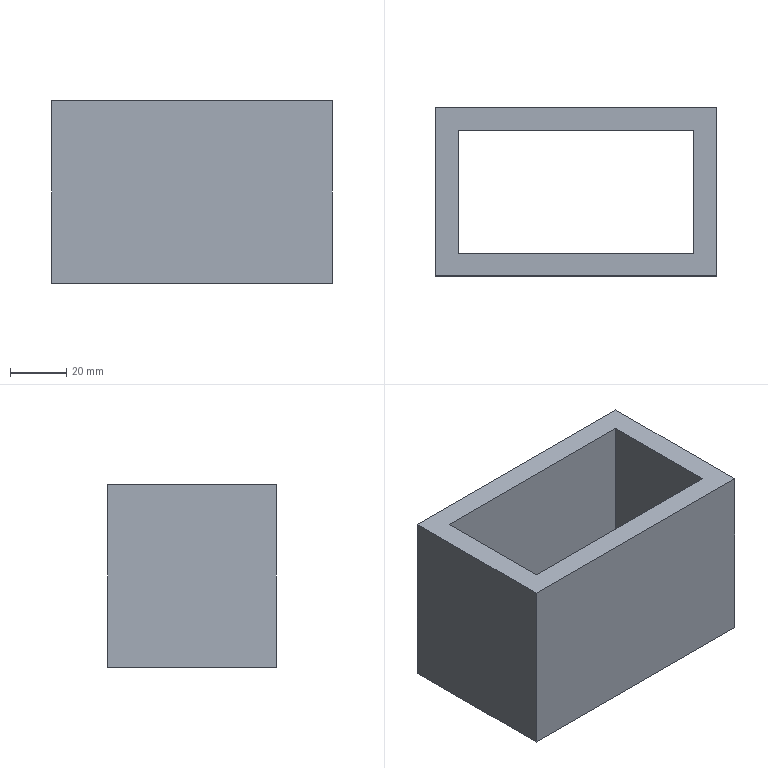Part | SolidWorks | features BaseBody 1 | 1 solid | 10 faces | box 100 x 60 x 65 mm | volume 149760 mm3 | plane 10
STEP:
#1=CARTESIAN_POINT('',(-50.,-30.,32.5));
#2=VERTEX_POINT('',#1);
#3=CARTESIAN_POINT('',(50.,-30.,32.5));
#4=VERTEX_POINT('',#3);
#5=CARTESIAN_POINT('',(-50.,-30.,32.5));
#6=DIRECTION('',(1.,0.,0.));
#7=VECTOR('',#6,1000.);
#8=LINE('',#5,#7);
#9=EDGE_CURVE('',#2,#4,#8,.T.);
#10=ORIENTED_EDGE('',*,*,#9,.F.);
#11=CARTESIAN_POINT('',(-50.,-30.,-32.5));
#12=VERTEX_POINT('',#11);
#13=CARTESIAN_POINT('',(-50.,-30.,-32.5));
#14=DIRECTION('',(0.,0.,1.));
#15=VECTOR('',#14,1000.);
#16=LINE('',#13,#15);
#17=EDGE_CURVE('',#12,#2,#16,.T.);
#18=ORIENTED_EDGE('',*,*,#17,.F.);
#19=CARTESIAN_POINT('',(50.,-30.,-32.5));
#20=VERTEX_POINT('',#19);
#21=CARTESIAN_POINT('',(-50.,-30.,-32.5));
#22=DIRECTION('',(-1.,0.,0.));
#23=VECTOR('',#22,1000.);
#24=LINE('',#21,#23);
#25=EDGE_CURVE('',#20,#12,#24,.T.);
#26=ORIENTED_EDGE('',*,*,#25,.F.);
#27=CARTESIAN_POINT('',(50.,-30.,-32.5));
#28=DIRECTION('',(0.,0.,-1.));
#29=VECTOR('',#28,1000.);
#30=LINE('',#27,#29);
#31=EDGE_CURVE('',#4,#20,#30,.T.);
#32=ORIENTED_EDGE('',*,*,#31,.F.);
#33=EDGE_LOOP('',(#10,#18,#26,#32));
#34=FACE_OUTER_BOUND('',#33,.T.);
#35=CARTESIAN_POINT('',(-50.,-30.,-32.5));
#36=DIRECTION('',(0.,1.,0.));
#37=DIRECTION('',(0.,0.,1.));
#38=AXIS2_PLACEMENT_3D('',#35,#36,#37);
#39=PLANE('',#38);
#40=ADVANCED_FACE('',(#34),#39,.F.);
#41=CARTESIAN_POINT('',(50.,30.,-32.5));
#42=VERTEX_POINT('',#41);
#43=CARTESIAN_POINT('',(50.,30.,32.5));
#44=VERTEX_POINT('',#43);
#45=CARTESIAN_POINT('',(50.,30.,-32.5));
#46=DIRECTION('',(0.,0.,1.));
#47=VECTOR('',#46,1000.);
#48=LINE('',#45,#47);
#49=EDGE_CURVE('',#42,#44,#48,.T.);
#50=ORIENTED_EDGE('',*,*,#49,.T.);
#51=CARTESIAN_POINT('',(50.,-30.,32.5));
#52=DIRECTION('',(0.,-1.,0.));
#53=VECTOR('',#52,1000.);
#54=LINE('',#51,#53);
#55=EDGE_CURVE('',#44,#4,#54,.T.);
#56=ORIENTED_EDGE('',*,*,#55,.T.);
#57=ORIENTED_EDGE('',*,*,#31,.T.);
#58=CARTESIAN_POINT('',(50.,-30.,-32.5));
#59=DIRECTION('',(0.,1.,0.));
#60=VECTOR('',#59,1000.);
#61=LINE('',#58,#60);
#62=EDGE_CURVE('',#20,#42,#61,.T.);
#63=ORIENTED_EDGE('',*,*,#62,.T.);
#64=EDGE_LOOP('',(#50,#56,#57,#63));
#65=FACE_OUTER_BOUND('',#64,.T.);
#66=CARTESIAN_POINT('',(50.,-30.,-32.5));
#67=DIRECTION('',(1.,0.,0.));
#68=DIRECTION('',(0.,0.,-1.));
#69=AXIS2_PLACEMENT_3D('',#66,#67,#68);
#70=PLANE('',#69);
#71=ADVANCED_FACE('',(#65),#70,.T.);
#72=CARTESIAN_POINT('',(-42.,22.,32.5));
#73=VERTEX_POINT('',#72);
#74=CARTESIAN_POINT('',(42.,22.,32.5));
#75=VERTEX_POINT('',#74);
#76=CARTESIAN_POINT('',(-50.,22.,32.5));
#77=DIRECTION('',(1.,0.,0.));
#78=VECTOR('',#77,1000.);
#79=LINE('',#76,#78);
#80=EDGE_CURVE('',#73,#75,#79,.T.);
#81=ORIENTED_EDGE('',*,*,#80,.T.);
#82=CARTESIAN_POINT('',(42.,-22.,32.5));
#83=VERTEX_POINT('',#82);
#84=CARTESIAN_POINT('',(42.,-30.,32.5));
#85=DIRECTION('',(0.,-1.,0.));
#86=VECTOR('',#85,1000.);
#87=LINE('',#84,#86);
#88=EDGE_CURVE('',#75,#83,#87,.T.);
#89=ORIENTED_EDGE('',*,*,#88,.T.);
#90=CARTESIAN_POINT('',(-42.,-22.,32.5));
#91=VERTEX_POINT('',#90);
#92=CARTESIAN_POINT('',(-50.,-22.,32.5));
#93=DIRECTION('',(-1.,0.,0.));
#94=VECTOR('',#93,1000.);
#95=LINE('',#92,#94);
#96=EDGE_CURVE('',#83,#91,#95,.T.);
#97=ORIENTED_EDGE('',*,*,#96,.T.);
#98=CARTESIAN_POINT('',(-42.,-30.,32.5));
#99=DIRECTION('',(0.,1.,0.));
#100=VECTOR('',#99,1000.);
#101=LINE('',#98,#100);
#102=EDGE_CURVE('',#91,#73,#101,.T.);
#103=ORIENTED_EDGE('',*,*,#102,.T.);
#104=EDGE_LOOP('',(#81,#89,#97,#103));
#105=FACE_BOUND('',#104,.T.);
#106=ORIENTED_EDGE('',*,*,#55,.F.);
#107=CARTESIAN_POINT('',(-50.,30.,32.5));
#108=VERTEX_POINT('',#107);
#109=CARTESIAN_POINT('',(-50.,30.,32.5));
#110=DIRECTION('',(-1.,0.,0.));
#111=VECTOR('',#110,1000.);
#112=LINE('',#109,#111);
#113=EDGE_CURVE('',#44,#108,#112,.T.);
#114=ORIENTED_EDGE('',*,*,#113,.T.);
#115=CARTESIAN_POINT('',(-50.,-30.,32.5));
#116=DIRECTION('',(0.,-1.,0.));
#117=VECTOR('',#116,1000.);
#118=LINE('',#115,#117);
#119=EDGE_CURVE('',#108,#2,#118,.T.);
#120=ORIENTED_EDGE('',*,*,#119,.T.);
#121=ORIENTED_EDGE('',*,*,#9,.T.);
#122=EDGE_LOOP('',(#106,#114,#120,#121));
#123=FACE_OUTER_BOUND('',#122,.T.);
#124=CARTESIAN_POINT('',(-50.,-30.,32.5));
#125=DIRECTION('',(0.,0.,1.));
#126=DIRECTION('',(1.,0.,0.));
#127=AXIS2_PLACEMENT_3D('',#124,#125,#126);
#128=PLANE('',#127);
#129=ADVANCED_FACE('',(#105,#123),#128,.T.);
#130=CARTESIAN_POINT('',(-50.,30.,-32.5));
#131=VERTEX_POINT('',#130);
#132=CARTESIAN_POINT('',(-50.,30.,-32.5));
#133=DIRECTION('',(0.,0.,1.));
#134=VECTOR('',#133,1000.);
#135=LINE('',#132,#134);
#136=EDGE_CURVE('',#131,#108,#135,.T.);
#137=ORIENTED_EDGE('',*,*,#136,.F.);
#138=CARTESIAN_POINT('',(-50.,-30.,-32.5));
#139=DIRECTION('',(0.,1.,0.));
#140=VECTOR('',#139,1000.);
#141=LINE('',#138,#140);
#142=EDGE_CURVE('',#12,#131,#141,.T.);
#143=ORIENTED_EDGE('',*,*,#142,.F.);
#144=ORIENTED_EDGE('',*,*,#17,.T.);
#145=ORIENTED_EDGE('',*,*,#119,.F.);
#146=EDGE_LOOP('',(#137,#143,#144,#145));
#147=FACE_OUTER_BOUND('',#146,.T.);
#148=CARTESIAN_POINT('',(-50.,-30.,-32.5));
#149=DIRECTION('',(1.,0.,0.));
#150=DIRECTION('',(0.,0.,-1.));
#151=AXIS2_PLACEMENT_3D('',#148,#149,#150);
#152=PLANE('',#151);
#153=ADVANCED_FACE('',(#147),#152,.F.);
#154=CARTESIAN_POINT('',(-42.,22.,-32.5));
#155=VERTEX_POINT('',#154);
#156=CARTESIAN_POINT('',(42.,22.,-32.5));
#157=VERTEX_POINT('',#156);
#158=CARTESIAN_POINT('',(-50.,22.,-32.5));
#159=DIRECTION('',(1.,0.,0.));
#160=VECTOR('',#159,1000.);
#161=LINE('',#158,#160);
#162=EDGE_CURVE('',#155,#157,#161,.T.);
#163=ORIENTED_EDGE('',*,*,#162,.F.);
#164=CARTESIAN_POINT('',(-42.,-22.,-32.5));
#165=VERTEX_POINT('',#164);
#166=CARTESIAN_POINT('',(-42.,-30.,-32.5));
#167=DIRECTION('',(0.,1.,0.));
#168=VECTOR('',#167,1000.);
#169=LINE('',#166,#168);
#170=EDGE_CURVE('',#165,#155,#169,.T.);
#171=ORIENTED_EDGE('',*,*,#170,.F.);
#172=CARTESIAN_POINT('',(42.,-22.,-32.5));
#173=VERTEX_POINT('',#172);
#174=CARTESIAN_POINT('',(-50.,-22.,-32.5));
#175=DIRECTION('',(-1.,0.,0.));
#176=VECTOR('',#175,1000.);
#177=LINE('',#174,#176);
#178=EDGE_CURVE('',#173,#165,#177,.T.);
#179=ORIENTED_EDGE('',*,*,#178,.F.);
#180=CARTESIAN_POINT('',(42.,-30.,-32.5));
#181=DIRECTION('',(0.,-1.,0.));
#182=VECTOR('',#181,1000.);
#183=LINE('',#180,#182);
#184=EDGE_CURVE('',#157,#173,#183,.T.);
#185=ORIENTED_EDGE('',*,*,#184,.F.);
#186=EDGE_LOOP('',(#163,#171,#179,#185));
#187=FACE_BOUND('',#186,.T.);
#188=ORIENTED_EDGE('',*,*,#62,.F.);
#189=ORIENTED_EDGE('',*,*,#25,.T.);
#190=ORIENTED_EDGE('',*,*,#142,.T.);
#191=CARTESIAN_POINT('',(-50.,30.,-32.5));
#192=DIRECTION('',(-1.,0.,0.));
#193=VECTOR('',#192,1000.);
#194=LINE('',#191,#193);
#195=EDGE_CURVE('',#42,#131,#194,.T.);
#196=ORIENTED_EDGE('',*,*,#195,.F.);
#197=EDGE_LOOP('',(#188,#189,#190,#196));
#198=FACE_OUTER_BOUND('',#197,.T.);
#199=CARTESIAN_POINT('',(-50.,-30.,-32.5));
#200=DIRECTION('',(0.,0.,1.));
#201=DIRECTION('',(1.,0.,0.));
#202=AXIS2_PLACEMENT_3D('',#199,#200,#201);
#203=PLANE('',#202);
#204=ADVANCED_FACE('',(#187,#198),#203,.F.);
#205=ORIENTED_EDGE('',*,*,#113,.F.);
#206=ORIENTED_EDGE('',*,*,#49,.F.);
#207=ORIENTED_EDGE('',*,*,#195,.T.);
#208=ORIENTED_EDGE('',*,*,#136,.T.);
#209=EDGE_LOOP('',(#205,#206,#207,#208));
#210=FACE_OUTER_BOUND('',#209,.T.);
#211=CARTESIAN_POINT('',(-50.,30.,-32.5));
#212=DIRECTION('',(0.,1.,0.));
#213=DIRECTION('',(0.,0.,1.));
#214=AXIS2_PLACEMENT_3D('',#211,#212,#213);
#215=PLANE('',#214);
#216=ADVANCED_FACE('',(#210),#215,.T.);
#217=CARTESIAN_POINT('',(42.,22.,-33.5));
#218=DIRECTION('',(0.,0.,1.));
#219=VECTOR('',#218,1000.);
#220=LINE('',#217,#219);
#221=EDGE_CURVE('',#157,#75,#220,.T.);
#222=ORIENTED_EDGE('',*,*,#221,.F.);
#223=ORIENTED_EDGE('',*,*,#184,.T.);
#224=CARTESIAN_POINT('',(42.,-22.,-33.5));
#225=DIRECTION('',(0.,0.,-1.));
#226=VECTOR('',#225,1000.);
#227=LINE('',#224,#226);
#228=EDGE_CURVE('',#83,#173,#227,.T.);
#229=ORIENTED_EDGE('',*,*,#228,.F.);
#230=ORIENTED_EDGE('',*,*,#88,.F.);
#231=EDGE_LOOP('',(#222,#223,#229,#230));
#232=FACE_OUTER_BOUND('',#231,.T.);
#233=CARTESIAN_POINT('',(42.,-22.,-33.5));
#234=DIRECTION('',(1.,0.,0.));
#235=DIRECTION('',(0.,0.,-1.));
#236=AXIS2_PLACEMENT_3D('',#233,#234,#235);
#237=PLANE('',#236);
#238=ADVANCED_FACE('',(#232),#237,.F.);
#239=CARTESIAN_POINT('',(-42.,22.,-33.5));
#240=DIRECTION('',(0.,0.,1.));
#241=VECTOR('',#240,1000.);
#242=LINE('',#239,#241);
#243=EDGE_CURVE('',#155,#73,#242,.T.);
#244=ORIENTED_EDGE('',*,*,#243,.F.);
#245=ORIENTED_EDGE('',*,*,#162,.T.);
#246=ORIENTED_EDGE('',*,*,#221,.T.);
#247=ORIENTED_EDGE('',*,*,#80,.F.);
#248=EDGE_LOOP('',(#244,#245,#246,#247));
#249=FACE_OUTER_BOUND('',#248,.T.);
#250=CARTESIAN_POINT('',(-42.,22.,-33.5));
#251=DIRECTION('',(0.,1.,0.));
#252=DIRECTION('',(0.,0.,1.));
#253=AXIS2_PLACEMENT_3D('',#250,#251,#252);
#254=PLANE('',#253);
#255=ADVANCED_FACE('',(#249),#254,.F.);
#256=ORIENTED_EDGE('',*,*,#243,.T.);
#257=ORIENTED_EDGE('',*,*,#102,.F.);
#258=CARTESIAN_POINT('',(-42.,-22.,-33.5));
#259=DIRECTION('',(0.,0.,-1.));
#260=VECTOR('',#259,1000.);
#261=LINE('',#258,#260);
#262=EDGE_CURVE('',#91,#165,#261,.T.);
#263=ORIENTED_EDGE('',*,*,#262,.T.);
#264=ORIENTED_EDGE('',*,*,#170,.T.);
#265=EDGE_LOOP('',(#256,#257,#263,#264));
#266=FACE_OUTER_BOUND('',#265,.T.);
#267=CARTESIAN_POINT('',(-42.,-22.,-33.5));
#268=DIRECTION('',(1.,0.,0.));
#269=DIRECTION('',(0.,0.,-1.));
#270=AXIS2_PLACEMENT_3D('',#267,#268,#269);
#271=PLANE('',#270);
#272=ADVANCED_FACE('',(#266),#271,.T.);
#273=ORIENTED_EDGE('',*,*,#262,.F.);
#274=ORIENTED_EDGE('',*,*,#96,.F.);
#275=ORIENTED_EDGE('',*,*,#228,.T.);
#276=ORIENTED_EDGE('',*,*,#178,.T.);
#277=EDGE_LOOP('',(#273,#274,#275,#276));
#278=FACE_OUTER_BOUND('',#277,.T.);
#279=CARTESIAN_POINT('',(-42.,-22.,-33.5));
#280=DIRECTION('',(0.,1.,0.));
#281=DIRECTION('',(0.,0.,1.));
#282=AXIS2_PLACEMENT_3D('',#279,#280,#281);
#283=PLANE('',#282);
#284=ADVANCED_FACE('',(#278),#283,.T.);
#285=CLOSED_SHELL('',(#40,#71,#129,#153,#204,#216,#238,#255,#272,#284));
#286=MANIFOLD_SOLID_BREP('',#285);
#287=CARTESIAN_POINT('',(0.,0.,0.));
#288=DIRECTION('',(0.,0.,1.));
#289=DIRECTION('',(1.,0.,0.));
#290=AXIS2_PLACEMENT_3D('',#287,#288,#289);
#291=(LENGTH_UNIT()NAMED_UNIT(*)SI_UNIT(.MILLI.,.METRE.));
#292=UNCERTAINTY_MEASURE_WITH_UNIT(LENGTH_MEASURE(0.00001),#291,'','');
#293=(NAMED_UNIT(*)PLANE_ANGLE_UNIT()SI_UNIT($,.RADIAN.));
#294=(NAMED_UNIT(*)SI_UNIT($,.STERADIAN.)SOLID_ANGLE_UNIT());
#295=(GEOMETRIC_REPRESENTATION_CONTEXT(3)GLOBAL_UNCERTAINTY_ASSIGNED_CONTEXT((#292))GLOBAL_UNIT_ASSIGNED_CONTEXT((#291,#293,#294))REPRESENTATION_CONTEXT('',''));
#296=ADVANCED_BREP_SHAPE_REPRESENTATION('',(#286,#290),#295);